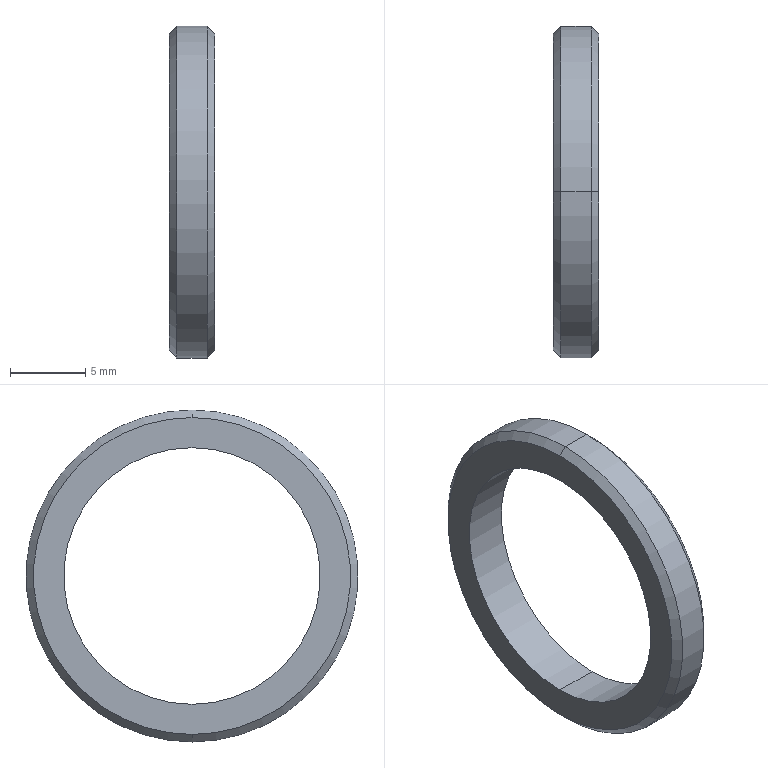Part | STEP file | 0245_002_CLBUM17-22-3 | 1 solid | 10 faces | box 3 x 22 x 22 mm | volume 442.441 mm3 | cone 4 | cylinder 4 | plane 2 | commonest cylinder face diameters 17 x2 22 x2
STEP:
#1=CARTESIAN_POINT('',(0.,0.,0.));
#2=DIRECTION('',(0.,0.,1.));
#3=DIRECTION('',(1.,0.,0.));
#4=AXIS2_PLACEMENT_3D('',#1,#2,#3);
#5=CARTESIAN_POINT('',(0.,0.,10.5));
#6=VERTEX_POINT('',#5);
#7=CARTESIAN_POINT('',(0.,0.,-10.5));
#8=VERTEX_POINT('',#7);
#9=CARTESIAN_POINT('',(0.,0.,0.));
#10=DIRECTION('',(-1.,0.,0.));
#11=DIRECTION('',(0.,0.,-1.));
#12=AXIS2_PLACEMENT_3D('',#9,#10,#11);
#13=CIRCLE('',#12,10.5);
#14=CARTESIAN_POINT('',(0.5,0.,0.));
#15=DIRECTION('',(1.,0.,0.));
#16=DIRECTION('',(0.,0.,-1.));
#17=AXIS2_PLACEMENT_3D('',#14,#15,#16);
#18=CONICAL_SURFACE('',#17,11.,0.7854);
#19=CARTESIAN_POINT('',(6.283,-0.5));
#20=DIRECTION('',(-1.,0.));
#21=VECTOR('',#20,1.);
#22=LINE('',#19,#21);
#23=(GEOMETRIC_REPRESENTATION_CONTEXT(2)PARAMETRIC_REPRESENTATION_CONTEXT()REPRESENTATION_CONTEXT('',''));
#24=DEFINITIONAL_REPRESENTATION('',(#22),#23);
#25=PCURVE('',#18,#24);
#26=CARTESIAN_POINT('',(0.,9.5,0.));
#27=DIRECTION('',(-1.,0.,0.));
#28=DIRECTION('',(0.,0.,1.));
#29=AXIS2_PLACEMENT_3D('',#26,#27,#28);
#30=PLANE('',#29);
#31=CARTESIAN_POINT('',(0.,-9.5));
#32=DIRECTION('',(-1.,0.));
#33=AXIS2_PLACEMENT_2D('',#31,#32);
#34=CIRCLE('',#33,10.5);
#35=(GEOMETRIC_REPRESENTATION_CONTEXT(2)PARAMETRIC_REPRESENTATION_CONTEXT()REPRESENTATION_CONTEXT('',''));
#36=DEFINITIONAL_REPRESENTATION('',(#34),#35);
#37=PCURVE('',#30,#36);
#38=SURFACE_CURVE('',#13,(#25,#37),.PCURVE_S1.);
#39=EDGE_CURVE('',#6,#8,#38,.T.);
#40=ORIENTED_EDGE('',*,*,#39,.F.);
#41=CARTESIAN_POINT('',(0.5,0.,11.));
#42=VERTEX_POINT('',#41);
#43=CARTESIAN_POINT('',(0.5,0.,11.));
#44=DIRECTION('',(0.7071,0.,0.7071));
#45=VECTOR('',#44,1.);
#46=LINE('',#43,#45);
#47=CARTESIAN_POINT('',(3.142,0.));
#48=DIRECTION('',(0.,1.));
#49=VECTOR('',#48,1.);
#50=LINE('',#47,#49);
#51=(GEOMETRIC_REPRESENTATION_CONTEXT(2)PARAMETRIC_REPRESENTATION_CONTEXT()REPRESENTATION_CONTEXT('',''));
#52=DEFINITIONAL_REPRESENTATION('',(#50),#51);
#53=PCURVE('',#18,#52);
#54=CARTESIAN_POINT('',(0.5,0.,0.));
#55=DIRECTION('',(1.,0.,0.));
#56=DIRECTION('',(0.,0.,-1.));
#57=AXIS2_PLACEMENT_3D('',#54,#55,#56);
#58=CONICAL_SURFACE('',#57,11.,0.7854);
#59=CARTESIAN_POINT('',(3.142,0.));
#60=DIRECTION('',(0.,1.));
#61=VECTOR('',#60,1.);
#62=LINE('',#59,#61);
#63=(GEOMETRIC_REPRESENTATION_CONTEXT(2)PARAMETRIC_REPRESENTATION_CONTEXT()REPRESENTATION_CONTEXT('',''));
#64=DEFINITIONAL_REPRESENTATION('',(#62),#63);
#65=PCURVE('',#58,#64);
#66=SURFACE_CURVE('',#46,(#53,#65),.PCURVE_S1.);
#67=EDGE_CURVE('',#6,#42,#66,.T.);
#68=ORIENTED_EDGE('',*,*,#67,.T.);
#69=CARTESIAN_POINT('',(0.5,0.,-11.));
#70=VERTEX_POINT('',#69);
#71=CARTESIAN_POINT('',(0.5,0.,0.));
#72=DIRECTION('',(-1.,0.,0.));
#73=DIRECTION('',(0.,1.,0.));
#74=AXIS2_PLACEMENT_3D('',#71,#72,#73);
#75=CIRCLE('',#74,11.);
#76=CARTESIAN_POINT('',(7.854,0.));
#77=DIRECTION('',(-1.,0.));
#78=VECTOR('',#77,1.);
#79=LINE('',#76,#78);
#80=(GEOMETRIC_REPRESENTATION_CONTEXT(2)PARAMETRIC_REPRESENTATION_CONTEXT()REPRESENTATION_CONTEXT('',''));
#81=DEFINITIONAL_REPRESENTATION('',(#79),#80);
#82=PCURVE('',#18,#81);
#83=CARTESIAN_POINT('',(1.5,0.,0.));
#84=DIRECTION('',(1.,0.,0.));
#85=DIRECTION('',(0.,0.,-1.));
#86=AXIS2_PLACEMENT_3D('',#83,#84,#85);
#87=CYLINDRICAL_SURFACE('',#86,11.);
#88=CARTESIAN_POINT('',(7.854,-1.));
#89=DIRECTION('',(-1.,0.));
#90=VECTOR('',#89,1.);
#91=LINE('',#88,#90);
#92=(GEOMETRIC_REPRESENTATION_CONTEXT(2)PARAMETRIC_REPRESENTATION_CONTEXT()REPRESENTATION_CONTEXT('',''));
#93=DEFINITIONAL_REPRESENTATION('',(#91),#92);
#94=PCURVE('',#87,#93);
#95=SURFACE_CURVE('',#75,(#82,#94),.PCURVE_S1.);
#96=EDGE_CURVE('',#42,#70,#95,.T.);
#97=ORIENTED_EDGE('',*,*,#96,.T.);
#98=CARTESIAN_POINT('',(0.5,0.,-11.));
#99=DIRECTION('',(0.7071,0.,-0.7071));
#100=VECTOR('',#99,1.);
#101=LINE('',#98,#100);
#102=CARTESIAN_POINT('',(0.,0.));
#103=DIRECTION('',(0.,1.));
#104=VECTOR('',#103,1.);
#105=LINE('',#102,#104);
#106=(GEOMETRIC_REPRESENTATION_CONTEXT(2)PARAMETRIC_REPRESENTATION_CONTEXT()REPRESENTATION_CONTEXT('',''));
#107=DEFINITIONAL_REPRESENTATION('',(#105),#106);
#108=PCURVE('',#18,#107);
#109=CARTESIAN_POINT('',(6.283,0.));
#110=DIRECTION('',(0.,1.));
#111=VECTOR('',#110,1.);
#112=LINE('',#109,#111);
#113=(GEOMETRIC_REPRESENTATION_CONTEXT(2)PARAMETRIC_REPRESENTATION_CONTEXT()REPRESENTATION_CONTEXT('',''));
#114=DEFINITIONAL_REPRESENTATION('',(#112),#113);
#115=PCURVE('',#58,#114);
#116=SURFACE_CURVE('',#101,(#108,#115),.PCURVE_S1.);
#117=EDGE_CURVE('',#8,#70,#116,.T.);
#118=ORIENTED_EDGE('',*,*,#117,.F.);
#119=EDGE_LOOP('',(#40,#68,#97,#118));
#120=FACE_BOUND('',#119,.T.);
#121=ADVANCED_FACE('',(#120),#18,.T.);
#122=CARTESIAN_POINT('',(0.,0.,-8.5));
#123=VERTEX_POINT('',#122);
#124=CARTESIAN_POINT('',(3.,0.,-8.5));
#125=VERTEX_POINT('',#124);
#126=CARTESIAN_POINT('',(1.5,0.,-8.5));
#127=DIRECTION('',(1.,0.,0.));
#128=VECTOR('',#127,1.);
#129=LINE('',#126,#128);
#130=CARTESIAN_POINT('',(1.5,0.,0.));
#131=DIRECTION('',(1.,0.,0.));
#132=DIRECTION('',(0.,0.,-1.));
#133=AXIS2_PLACEMENT_3D('',#130,#131,#132);
#134=CYLINDRICAL_SURFACE('',#133,8.5);
#135=CARTESIAN_POINT('',(6.283,0.));
#136=DIRECTION('',(0.,1.));
#137=VECTOR('',#136,1.);
#138=LINE('',#135,#137);
#139=(GEOMETRIC_REPRESENTATION_CONTEXT(2)PARAMETRIC_REPRESENTATION_CONTEXT()REPRESENTATION_CONTEXT('',''));
#140=DEFINITIONAL_REPRESENTATION('',(#138),#139);
#141=PCURVE('',#134,#140);
#142=CARTESIAN_POINT('',(1.5,0.,0.));
#143=DIRECTION('',(1.,0.,0.));
#144=DIRECTION('',(0.,0.,-1.));
#145=AXIS2_PLACEMENT_3D('',#142,#143,#144);
#146=CYLINDRICAL_SURFACE('',#145,8.5);
#147=CARTESIAN_POINT('',(0.,0.));
#148=DIRECTION('',(0.,1.));
#149=VECTOR('',#148,1.);
#150=LINE('',#147,#149);
#151=(GEOMETRIC_REPRESENTATION_CONTEXT(2)PARAMETRIC_REPRESENTATION_CONTEXT()REPRESENTATION_CONTEXT('',''));
#152=DEFINITIONAL_REPRESENTATION('',(#150),#151);
#153=PCURVE('',#146,#152);
#154=SURFACE_CURVE('',#129,(#141,#153),.PCURVE_S1.);
#155=EDGE_CURVE('',#123,#125,#154,.T.);
#156=ORIENTED_EDGE('',*,*,#155,.T.);
#157=CARTESIAN_POINT('',(3.,0.,8.5));
#158=VERTEX_POINT('',#157);
#159=CARTESIAN_POINT('',(3.,0.,0.));
#160=DIRECTION('',(-1.,0.,0.));
#161=DIRECTION('',(0.,0.,-1.));
#162=AXIS2_PLACEMENT_3D('',#159,#160,#161);
#163=CIRCLE('',#162,8.5);
#164=CARTESIAN_POINT('',(6.283,1.5));
#165=DIRECTION('',(-1.,0.));
#166=VECTOR('',#165,1.);
#167=LINE('',#164,#166);
#168=(GEOMETRIC_REPRESENTATION_CONTEXT(2)PARAMETRIC_REPRESENTATION_CONTEXT()REPRESENTATION_CONTEXT('',''));
#169=DEFINITIONAL_REPRESENTATION('',(#167),#168);
#170=PCURVE('',#134,#169);
#171=CARTESIAN_POINT('',(3.,9.5,0.));
#172=DIRECTION('',(1.,0.,0.));
#173=DIRECTION('',(0.,0.,-1.));
#174=AXIS2_PLACEMENT_3D('',#171,#172,#173);
#175=PLANE('',#174);
#176=CARTESIAN_POINT('',(8.5,-9.5));
#177=CARTESIAN_POINT('',(8.5,-24.222));
#178=CARTESIAN_POINT('',(-4.25,-16.861));
#179=CARTESIAN_POINT('',(-17.,-9.5));
#180=CARTESIAN_POINT('',(-4.25,-2.139));
#181=CARTESIAN_POINT('',(8.5,5.222));
#182=CARTESIAN_POINT('',(8.5,-9.5));
#183=(BOUNDED_CURVE()B_SPLINE_CURVE(2,(#176,#177,#178,#179,#180,#181,#182),.UNSPECIFIED.,.T.,.F.)B_SPLINE_CURVE_WITH_KNOTS((1,2,2,2,2,1),(-2.094,0.,2.094,4.189,6.283,8.378),.UNSPECIFIED.)CURVE()GEOMETRIC_REPRESENTATION_ITEM()RATIONAL_B_SPLINE_CURVE((1.,0.5,1.,0.5,1.,0.5,1.))REPRESENTATION_ITEM(''));
#184=(GEOMETRIC_REPRESENTATION_CONTEXT(2)PARAMETRIC_REPRESENTATION_CONTEXT()REPRESENTATION_CONTEXT('',''));
#185=DEFINITIONAL_REPRESENTATION('',(#183),#184);
#186=PCURVE('',#175,#185);
#187=SURFACE_CURVE('',#163,(#170,#186),.PCURVE_S1.);
#188=EDGE_CURVE('',#125,#158,#187,.T.);
#189=ORIENTED_EDGE('',*,*,#188,.T.);
#190=CARTESIAN_POINT('',(0.,0.,8.5));
#191=VERTEX_POINT('',#190);
#192=CARTESIAN_POINT('',(1.5,0.,8.5));
#193=DIRECTION('',(1.,0.,0.));
#194=VECTOR('',#193,1.);
#195=LINE('',#192,#194);
#196=CARTESIAN_POINT('',(3.142,0.));
#197=DIRECTION('',(0.,1.));
#198=VECTOR('',#197,1.);
#199=LINE('',#196,#198);
#200=(GEOMETRIC_REPRESENTATION_CONTEXT(2)PARAMETRIC_REPRESENTATION_CONTEXT()REPRESENTATION_CONTEXT('',''));
#201=DEFINITIONAL_REPRESENTATION('',(#199),#200);
#202=PCURVE('',#134,#201);
#203=CARTESIAN_POINT('',(3.142,0.));
#204=DIRECTION('',(0.,1.));
#205=VECTOR('',#204,1.);
#206=LINE('',#203,#205);
#207=(GEOMETRIC_REPRESENTATION_CONTEXT(2)PARAMETRIC_REPRESENTATION_CONTEXT()REPRESENTATION_CONTEXT('',''));
#208=DEFINITIONAL_REPRESENTATION('',(#206),#207);
#209=PCURVE('',#146,#208);
#210=SURFACE_CURVE('',#195,(#202,#209),.PCURVE_S1.);
#211=EDGE_CURVE('',#191,#158,#210,.T.);
#212=ORIENTED_EDGE('',*,*,#211,.F.);
#213=CARTESIAN_POINT('',(0.,0.,0.));
#214=DIRECTION('',(1.,0.,0.));
#215=DIRECTION('',(0.,0.,-1.));
#216=AXIS2_PLACEMENT_3D('',#213,#214,#215);
#217=CIRCLE('',#216,8.5);
#218=CARTESIAN_POINT('',(0.,-1.5));
#219=DIRECTION('',(1.,0.));
#220=VECTOR('',#219,1.);
#221=LINE('',#218,#220);
#222=(GEOMETRIC_REPRESENTATION_CONTEXT(2)PARAMETRIC_REPRESENTATION_CONTEXT()REPRESENTATION_CONTEXT('',''));
#223=DEFINITIONAL_REPRESENTATION('',(#221),#222);
#224=PCURVE('',#134,#223);
#225=CARTESIAN_POINT('',(-8.5,-9.5));
#226=CARTESIAN_POINT('',(-8.5,5.222));
#227=CARTESIAN_POINT('',(4.25,-2.139));
#228=CARTESIAN_POINT('',(17.,-9.5));
#229=CARTESIAN_POINT('',(4.25,-16.861));
#230=CARTESIAN_POINT('',(-8.5,-24.222));
#231=CARTESIAN_POINT('',(-8.5,-9.5));
#232=(BOUNDED_CURVE()B_SPLINE_CURVE(2,(#225,#226,#227,#228,#229,#230,#231),.UNSPECIFIED.,.T.,.F.)B_SPLINE_CURVE_WITH_KNOTS((1,2,2,2,2,1),(-2.094,0.,2.094,4.189,6.283,8.378),.UNSPECIFIED.)CURVE()GEOMETRIC_REPRESENTATION_ITEM()RATIONAL_B_SPLINE_CURVE((1.,0.5,1.,0.5,1.,0.5,1.))REPRESENTATION_ITEM(''));
#233=(GEOMETRIC_REPRESENTATION_CONTEXT(2)PARAMETRIC_REPRESENTATION_CONTEXT()REPRESENTATION_CONTEXT('',''));
#234=DEFINITIONAL_REPRESENTATION('',(#232),#233);
#235=PCURVE('',#30,#234);
#236=SURFACE_CURVE('',#217,(#224,#235),.PCURVE_S1.);
#237=EDGE_CURVE('',#191,#123,#236,.T.);
#238=ORIENTED_EDGE('',*,*,#237,.T.);
#239=EDGE_LOOP('',(#156,#189,#212,#238));
#240=FACE_BOUND('',#239,.F.);
#241=ADVANCED_FACE('',(#240),#134,.F.);
#242=ORIENTED_EDGE('',*,*,#96,.F.);
#243=CARTESIAN_POINT('',(2.5,0.,11.));
#244=VERTEX_POINT('',#243);
#245=CARTESIAN_POINT('',(1.5,0.,11.));
#246=DIRECTION('',(1.,0.,0.));
#247=VECTOR('',#246,1.);
#248=LINE('',#245,#247);
#249=CARTESIAN_POINT('',(3.142,0.));
#250=DIRECTION('',(0.,1.));
#251=VECTOR('',#250,1.);
#252=LINE('',#249,#251);
#253=(GEOMETRIC_REPRESENTATION_CONTEXT(2)PARAMETRIC_REPRESENTATION_CONTEXT()REPRESENTATION_CONTEXT('',''));
#254=DEFINITIONAL_REPRESENTATION('',(#252),#253);
#255=PCURVE('',#87,#254);
#256=CARTESIAN_POINT('',(1.5,0.,0.));
#257=DIRECTION('',(1.,0.,0.));
#258=DIRECTION('',(0.,0.,-1.));
#259=AXIS2_PLACEMENT_3D('',#256,#257,#258);
#260=CYLINDRICAL_SURFACE('',#259,11.);
#261=CARTESIAN_POINT('',(3.142,0.));
#262=DIRECTION('',(0.,1.));
#263=VECTOR('',#262,1.);
#264=LINE('',#261,#263);
#265=(GEOMETRIC_REPRESENTATION_CONTEXT(2)PARAMETRIC_REPRESENTATION_CONTEXT()REPRESENTATION_CONTEXT('',''));
#266=DEFINITIONAL_REPRESENTATION('',(#264),#265);
#267=PCURVE('',#260,#266);
#268=SURFACE_CURVE('',#248,(#255,#267),.PCURVE_S1.);
#269=EDGE_CURVE('',#42,#244,#268,.T.);
#270=ORIENTED_EDGE('',*,*,#269,.T.);
#271=CARTESIAN_POINT('',(2.5,0.,-11.));
#272=VERTEX_POINT('',#271);
#273=CARTESIAN_POINT('',(2.5,0.,0.));
#274=DIRECTION('',(-1.,0.,0.));
#275=DIRECTION('',(0.,0.,-1.));
#276=AXIS2_PLACEMENT_3D('',#273,#274,#275);
#277=CIRCLE('',#276,11.);
#278=CARTESIAN_POINT('',(6.283,1.));
#279=DIRECTION('',(-1.,0.));
#280=VECTOR('',#279,1.);
#281=LINE('',#278,#280);
#282=(GEOMETRIC_REPRESENTATION_CONTEXT(2)PARAMETRIC_REPRESENTATION_CONTEXT()REPRESENTATION_CONTEXT('',''));
#283=DEFINITIONAL_REPRESENTATION('',(#281),#282);
#284=PCURVE('',#87,#283);
#285=CARTESIAN_POINT('',(2.5,0.,0.));
#286=DIRECTION('',(-1.,0.,0.));
#287=DIRECTION('',(0.,0.,1.));
#288=AXIS2_PLACEMENT_3D('',#285,#286,#287);
#289=CONICAL_SURFACE('',#288,11.,0.7854);
#290=CARTESIAN_POINT('',(-3.142,0.));
#291=DIRECTION('',(1.,0.));
#292=VECTOR('',#291,1.);
#293=LINE('',#290,#292);
#294=(GEOMETRIC_REPRESENTATION_CONTEXT(2)PARAMETRIC_REPRESENTATION_CONTEXT()REPRESENTATION_CONTEXT('',''));
#295=DEFINITIONAL_REPRESENTATION('',(#293),#294);
#296=PCURVE('',#289,#295);
#297=SURFACE_CURVE('',#277,(#284,#296),.PCURVE_S1.);
#298=EDGE_CURVE('',#244,#272,#297,.T.);
#299=ORIENTED_EDGE('',*,*,#298,.T.);
#300=CARTESIAN_POINT('',(1.5,0.,-11.));
#301=DIRECTION('',(1.,0.,0.));
#302=VECTOR('',#301,1.);
#303=LINE('',#300,#302);
#304=CARTESIAN_POINT('',(0.,0.));
#305=DIRECTION('',(0.,1.));
#306=VECTOR('',#305,1.);
#307=LINE('',#304,#306);
#308=(GEOMETRIC_REPRESENTATION_CONTEXT(2)PARAMETRIC_REPRESENTATION_CONTEXT()REPRESENTATION_CONTEXT('',''));
#309=DEFINITIONAL_REPRESENTATION('',(#307),#308);
#310=PCURVE('',#87,#309);
#311=CARTESIAN_POINT('',(6.283,0.));
#312=DIRECTION('',(0.,1.));
#313=VECTOR('',#312,1.);
#314=LINE('',#311,#313);
#315=(GEOMETRIC_REPRESENTATION_CONTEXT(2)PARAMETRIC_REPRESENTATION_CONTEXT()REPRESENTATION_CONTEXT('',''));
#316=DEFINITIONAL_REPRESENTATION('',(#314),#315);
#317=PCURVE('',#260,#316);
#318=SURFACE_CURVE('',#303,(#310,#317),.PCURVE_S1.);
#319=EDGE_CURVE('',#70,#272,#318,.T.);
#320=ORIENTED_EDGE('',*,*,#319,.F.);
#321=EDGE_LOOP('',(#242,#270,#299,#320));
#322=FACE_BOUND('',#321,.T.);
#323=ADVANCED_FACE('',(#322),#87,.T.);
#324=CARTESIAN_POINT('',(3.,0.,-10.5));
#325=VERTEX_POINT('',#324);
#326=CARTESIAN_POINT('',(3.,0.,10.5));
#327=VERTEX_POINT('',#326);
#328=CARTESIAN_POINT('',(3.,0.,0.));
#329=DIRECTION('',(1.,0.,0.));
#330=DIRECTION('',(0.,0.,1.));
#331=AXIS2_PLACEMENT_3D('',#328,#329,#330);
#332=CIRCLE('',#331,10.5);
#333=CARTESIAN_POINT('',(6.283,-0.5));
#334=DIRECTION('',(-1.,0.));
#335=VECTOR('',#334,1.);
#336=LINE('',#333,#335);
#337=(GEOMETRIC_REPRESENTATION_CONTEXT(2)PARAMETRIC_REPRESENTATION_CONTEXT()REPRESENTATION_CONTEXT('',''));
#338=DEFINITIONAL_REPRESENTATION('',(#336),#337);
#339=PCURVE('',#289,#338);
#340=CARTESIAN_POINT('',(0.,-9.5));
#341=DIRECTION('',(-1.,0.));
#342=AXIS2_PLACEMENT_2D('',#340,#341);
#343=CIRCLE('',#342,10.5);
#344=(GEOMETRIC_REPRESENTATION_CONTEXT(2)PARAMETRIC_REPRESENTATION_CONTEXT()REPRESENTATION_CONTEXT('',''));
#345=DEFINITIONAL_REPRESENTATION('',(#343),#344);
#346=PCURVE('',#175,#345);
#347=SURFACE_CURVE('',#332,(#339,#346),.PCURVE_S1.);
#348=EDGE_CURVE('',#325,#327,#347,.T.);
#349=ORIENTED_EDGE('',*,*,#348,.F.);
#350=CARTESIAN_POINT('',(2.5,0.,-11.));
#351=DIRECTION('',(-0.7071,0.,-0.7071));
#352=VECTOR('',#351,1.);
#353=LINE('',#350,#352);
#354=CARTESIAN_POINT('',(3.142,0.));
#355=DIRECTION('',(0.,1.));
#356=VECTOR('',#355,1.);
#357=LINE('',#354,#356);
#358=(GEOMETRIC_REPRESENTATION_CONTEXT(2)PARAMETRIC_REPRESENTATION_CONTEXT()REPRESENTATION_CONTEXT('',''));
#359=DEFINITIONAL_REPRESENTATION('',(#357),#358);
#360=PCURVE('',#289,#359);
#361=CARTESIAN_POINT('',(2.5,0.,0.));
#362=DIRECTION('',(-1.,0.,0.));
#363=DIRECTION('',(0.,0.,1.));
#364=AXIS2_PLACEMENT_3D('',#361,#362,#363);
#365=CONICAL_SURFACE('',#364,11.,0.7854);
#366=CARTESIAN_POINT('',(3.142,0.));
#367=DIRECTION('',(0.,1.));
#368=VECTOR('',#367,1.);
#369=LINE('',#366,#368);
#370=(GEOMETRIC_REPRESENTATION_CONTEXT(2)PARAMETRIC_REPRESENTATION_CONTEXT()REPRESENTATION_CONTEXT('',''));
#371=DEFINITIONAL_REPRESENTATION('',(#369),#370);
#372=PCURVE('',#365,#371);
#373=SURFACE_CURVE('',#353,(#360,#372),.PCURVE_S1.);
#374=EDGE_CURVE('',#325,#272,#373,.T.);
#375=ORIENTED_EDGE('',*,*,#374,.T.);
#376=ORIENTED_EDGE('',*,*,#298,.F.);
#377=CARTESIAN_POINT('',(2.5,0.,11.));
#378=DIRECTION('',(-0.7071,0.,0.7071));
#379=VECTOR('',#378,1.);
#380=LINE('',#377,#379);
#381=CARTESIAN_POINT('',(0.,0.));
#382=DIRECTION('',(0.,1.));
#383=VECTOR('',#382,1.);
#384=LINE('',#381,#383);
#385=(GEOMETRIC_REPRESENTATION_CONTEXT(2)PARAMETRIC_REPRESENTATION_CONTEXT()REPRESENTATION_CONTEXT('',''));
#386=DEFINITIONAL_REPRESENTATION('',(#384),#385);
#387=PCURVE('',#289,#386);
#388=CARTESIAN_POINT('',(6.283,0.));
#389=DIRECTION('',(0.,1.));
#390=VECTOR('',#389,1.);
#391=LINE('',#388,#390);
#392=(GEOMETRIC_REPRESENTATION_CONTEXT(2)PARAMETRIC_REPRESENTATION_CONTEXT()REPRESENTATION_CONTEXT('',''));
#393=DEFINITIONAL_REPRESENTATION('',(#391),#392);
#394=PCURVE('',#365,#393);
#395=SURFACE_CURVE('',#380,(#387,#394),.PCURVE_S1.);
#396=EDGE_CURVE('',#327,#244,#395,.T.);
#397=ORIENTED_EDGE('',*,*,#396,.F.);
#398=EDGE_LOOP('',(#349,#375,#376,#397));
#399=FACE_BOUND('',#398,.T.);
#400=ADVANCED_FACE('',(#399),#289,.T.);
#401=CARTESIAN_POINT('',(0.,0.,0.));
#402=DIRECTION('',(-1.,0.,0.));
#403=DIRECTION('',(0.,0.,-1.));
#404=AXIS2_PLACEMENT_3D('',#401,#402,#403);
#405=CIRCLE('',#404,10.5);
#406=CARTESIAN_POINT('',(0.,-9.5));
#407=DIRECTION('',(-1.,0.));
#408=AXIS2_PLACEMENT_2D('',#406,#407);
#409=CIRCLE('',#408,10.5);
#410=(GEOMETRIC_REPRESENTATION_CONTEXT(2)PARAMETRIC_REPRESENTATION_CONTEXT()REPRESENTATION_CONTEXT('',''));
#411=DEFINITIONAL_REPRESENTATION('',(#409),#410);
#412=PCURVE('',#30,#411);
#413=CARTESIAN_POINT('',(6.283,-0.5));
#414=DIRECTION('',(-1.,0.));
#415=VECTOR('',#414,1.);
#416=LINE('',#413,#415);
#417=(GEOMETRIC_REPRESENTATION_CONTEXT(2)PARAMETRIC_REPRESENTATION_CONTEXT()REPRESENTATION_CONTEXT('',''));
#418=DEFINITIONAL_REPRESENTATION('',(#416),#417);
#419=PCURVE('',#58,#418);
#420=SURFACE_CURVE('',#405,(#412,#419),.PCURVE_S1.);
#421=EDGE_CURVE('',#8,#6,#420,.T.);
#422=ORIENTED_EDGE('',*,*,#421,.T.);
#423=ORIENTED_EDGE('',*,*,#39,.T.);
#424=EDGE_LOOP('',(#422,#423));
#425=FACE_BOUND('',#424,.T.);
#426=CARTESIAN_POINT('',(0.,0.,0.));
#427=DIRECTION('',(1.,0.,0.));
#428=DIRECTION('',(0.,0.,-1.));
#429=AXIS2_PLACEMENT_3D('',#426,#427,#428);
#430=CIRCLE('',#429,8.5);
#431=CARTESIAN_POINT('',(-8.5,-9.5));
#432=CARTESIAN_POINT('',(-8.5,5.222));
#433=CARTESIAN_POINT('',(4.25,-2.139));
#434=CARTESIAN_POINT('',(17.,-9.5));
#435=CARTESIAN_POINT('',(4.25,-16.861));
#436=CARTESIAN_POINT('',(-8.5,-24.222));
#437=CARTESIAN_POINT('',(-8.5,-9.5));
#438=(BOUNDED_CURVE()B_SPLINE_CURVE(2,(#431,#432,#433,#434,#435,#436,#437),.UNSPECIFIED.,.T.,.F.)B_SPLINE_CURVE_WITH_KNOTS((1,2,2,2,2,1),(-2.094,0.,2.094,4.189,6.283,8.378),.UNSPECIFIED.)CURVE()GEOMETRIC_REPRESENTATION_ITEM()RATIONAL_B_SPLINE_CURVE((1.,0.5,1.,0.5,1.,0.5,1.))REPRESENTATION_ITEM(''));
#439=(GEOMETRIC_REPRESENTATION_CONTEXT(2)PARAMETRIC_REPRESENTATION_CONTEXT()REPRESENTATION_CONTEXT('',''));
#440=DEFINITIONAL_REPRESENTATION('',(#438),#439);
#441=PCURVE('',#30,#440);
#442=CARTESIAN_POINT('',(0.,-1.5));
#443=DIRECTION('',(1.,0.));
#444=VECTOR('',#443,1.);
#445=LINE('',#442,#444);
#446=(GEOMETRIC_REPRESENTATION_CONTEXT(2)PARAMETRIC_REPRESENTATION_CONTEXT()REPRESENTATION_CONTEXT('',''));
#447=DEFINITIONAL_REPRESENTATION('',(#445),#446);
#448=PCURVE('',#146,#447);
#449=SURFACE_CURVE('',#430,(#441,#448),.PCURVE_S1.);
#450=EDGE_CURVE('',#123,#191,#449,.T.);
#451=ORIENTED_EDGE('',*,*,#450,.T.);
#452=ORIENTED_EDGE('',*,*,#237,.T.);
#453=EDGE_LOOP('',(#451,#452));
#454=FACE_BOUND('',#453,.T.);
#455=ADVANCED_FACE('',(#425,#454),#30,.T.);
#456=ORIENTED_EDGE('',*,*,#67,.F.);
#457=ORIENTED_EDGE('',*,*,#421,.F.);
#458=ORIENTED_EDGE('',*,*,#117,.T.);
#459=CARTESIAN_POINT('',(0.5,0.,0.));
#460=DIRECTION('',(-1.,0.,0.));
#461=DIRECTION('',(0.,1.,0.));
#462=AXIS2_PLACEMENT_3D('',#459,#460,#461);
#463=CIRCLE('',#462,11.);
#464=CARTESIAN_POINT('',(7.854,0.));
#465=DIRECTION('',(-1.,0.));
#466=VECTOR('',#465,1.);
#467=LINE('',#464,#466);
#468=(GEOMETRIC_REPRESENTATION_CONTEXT(2)PARAMETRIC_REPRESENTATION_CONTEXT()REPRESENTATION_CONTEXT('',''));
#469=DEFINITIONAL_REPRESENTATION('',(#467),#468);
#470=PCURVE('',#58,#469);
#471=CARTESIAN_POINT('',(7.854,-1.));
#472=DIRECTION('',(-1.,0.));
#473=VECTOR('',#472,1.);
#474=LINE('',#471,#473);
#475=(GEOMETRIC_REPRESENTATION_CONTEXT(2)PARAMETRIC_REPRESENTATION_CONTEXT()REPRESENTATION_CONTEXT('',''));
#476=DEFINITIONAL_REPRESENTATION('',(#474),#475);
#477=PCURVE('',#260,#476);
#478=SURFACE_CURVE('',#463,(#470,#477),.PCURVE_S1.);
#479=EDGE_CURVE('',#70,#42,#478,.T.);
#480=ORIENTED_EDGE('',*,*,#479,.T.);
#481=EDGE_LOOP('',(#456,#457,#458,#480));
#482=FACE_BOUND('',#481,.T.);
#483=ADVANCED_FACE('',(#482),#58,.T.);
#484=CARTESIAN_POINT('',(3.,0.,0.));
#485=DIRECTION('',(-1.,0.,0.));
#486=DIRECTION('',(0.,0.,-1.));
#487=AXIS2_PLACEMENT_3D('',#484,#485,#486);
#488=CIRCLE('',#487,8.5);
#489=CARTESIAN_POINT('',(6.283,1.5));
#490=DIRECTION('',(-1.,0.));
#491=VECTOR('',#490,1.);
#492=LINE('',#489,#491);
#493=(GEOMETRIC_REPRESENTATION_CONTEXT(2)PARAMETRIC_REPRESENTATION_CONTEXT()REPRESENTATION_CONTEXT('',''));
#494=DEFINITIONAL_REPRESENTATION('',(#492),#493);
#495=PCURVE('',#146,#494);
#496=CARTESIAN_POINT('',(8.5,-9.5));
#497=CARTESIAN_POINT('',(8.5,-24.222));
#498=CARTESIAN_POINT('',(-4.25,-16.861));
#499=CARTESIAN_POINT('',(-17.,-9.5));
#500=CARTESIAN_POINT('',(-4.25,-2.139));
#501=CARTESIAN_POINT('',(8.5,5.222));
#502=CARTESIAN_POINT('',(8.5,-9.5));
#503=(BOUNDED_CURVE()B_SPLINE_CURVE(2,(#496,#497,#498,#499,#500,#501,#502),.UNSPECIFIED.,.T.,.F.)B_SPLINE_CURVE_WITH_KNOTS((1,2,2,2,2,1),(-2.094,0.,2.094,4.189,6.283,8.378),.UNSPECIFIED.)CURVE()GEOMETRIC_REPRESENTATION_ITEM()RATIONAL_B_SPLINE_CURVE((1.,0.5,1.,0.5,1.,0.5,1.))REPRESENTATION_ITEM(''));
#504=(GEOMETRIC_REPRESENTATION_CONTEXT(2)PARAMETRIC_REPRESENTATION_CONTEXT()REPRESENTATION_CONTEXT('',''));
#505=DEFINITIONAL_REPRESENTATION('',(#503),#504);
#506=PCURVE('',#175,#505);
#507=SURFACE_CURVE('',#488,(#495,#506),.PCURVE_S1.);
#508=EDGE_CURVE('',#158,#125,#507,.T.);
#509=ORIENTED_EDGE('',*,*,#508,.T.);
#510=ORIENTED_EDGE('',*,*,#155,.F.);
#511=ORIENTED_EDGE('',*,*,#450,.T.);
#512=ORIENTED_EDGE('',*,*,#211,.T.);
#513=EDGE_LOOP('',(#509,#510,#511,#512));
#514=FACE_BOUND('',#513,.F.);
#515=ADVANCED_FACE('',(#514),#146,.F.);
#516=ORIENTED_EDGE('',*,*,#269,.F.);
#517=ORIENTED_EDGE('',*,*,#479,.F.);
#518=ORIENTED_EDGE('',*,*,#319,.T.);
#519=CARTESIAN_POINT('',(2.5,0.,0.));
#520=DIRECTION('',(-1.,0.,0.));
#521=DIRECTION('',(0.,0.,-1.));
#522=AXIS2_PLACEMENT_3D('',#519,#520,#521);
#523=CIRCLE('',#522,11.);
#524=CARTESIAN_POINT('',(6.283,1.));
#525=DIRECTION('',(-1.,0.));
#526=VECTOR('',#525,1.);
#527=LINE('',#524,#526);
#528=(GEOMETRIC_REPRESENTATION_CONTEXT(2)PARAMETRIC_REPRESENTATION_CONTEXT()REPRESENTATION_CONTEXT('',''));
#529=DEFINITIONAL_REPRESENTATION('',(#527),#528);
#530=PCURVE('',#260,#529);
#531=CARTESIAN_POINT('',(3.142,0.));
#532=DIRECTION('',(1.,0.));
#533=VECTOR('',#532,1.);
#534=LINE('',#531,#533);
#535=(GEOMETRIC_REPRESENTATION_CONTEXT(2)PARAMETRIC_REPRESENTATION_CONTEXT()REPRESENTATION_CONTEXT('',''));
#536=DEFINITIONAL_REPRESENTATION('',(#534),#535);
#537=PCURVE('',#365,#536);
#538=SURFACE_CURVE('',#523,(#530,#537),.PCURVE_S1.);
#539=EDGE_CURVE('',#272,#244,#538,.T.);
#540=ORIENTED_EDGE('',*,*,#539,.T.);
#541=EDGE_LOOP('',(#516,#517,#518,#540));
#542=FACE_BOUND('',#541,.T.);
#543=ADVANCED_FACE('',(#542),#260,.T.);
#544=ORIENTED_EDGE('',*,*,#188,.T.);
#545=ORIENTED_EDGE('',*,*,#508,.T.);
#546=EDGE_LOOP('',(#544,#545));
#547=FACE_BOUND('',#546,.T.);
#548=CARTESIAN_POINT('',(3.,0.,0.));
#549=DIRECTION('',(1.,0.,0.));
#550=DIRECTION('',(0.,0.,1.));
#551=AXIS2_PLACEMENT_3D('',#548,#549,#550);
#552=CIRCLE('',#551,10.5);
#553=CARTESIAN_POINT('',(0.,-9.5));
#554=DIRECTION('',(-1.,0.));
#555=AXIS2_PLACEMENT_2D('',#553,#554);
#556=CIRCLE('',#555,10.5);
#557=(GEOMETRIC_REPRESENTATION_CONTEXT(2)PARAMETRIC_REPRESENTATION_CONTEXT()REPRESENTATION_CONTEXT('',''));
#558=DEFINITIONAL_REPRESENTATION('',(#556),#557);
#559=PCURVE('',#175,#558);
#560=CARTESIAN_POINT('',(6.283,-0.5));
#561=DIRECTION('',(-1.,0.));
#562=VECTOR('',#561,1.);
#563=LINE('',#560,#562);
#564=(GEOMETRIC_REPRESENTATION_CONTEXT(2)PARAMETRIC_REPRESENTATION_CONTEXT()REPRESENTATION_CONTEXT('',''));
#565=DEFINITIONAL_REPRESENTATION('',(#563),#564);
#566=PCURVE('',#365,#565);
#567=SURFACE_CURVE('',#552,(#559,#566),.PCURVE_S1.);
#568=EDGE_CURVE('',#327,#325,#567,.T.);
#569=ORIENTED_EDGE('',*,*,#568,.T.);
#570=ORIENTED_EDGE('',*,*,#348,.T.);
#571=EDGE_LOOP('',(#569,#570));
#572=FACE_BOUND('',#571,.T.);
#573=ADVANCED_FACE('',(#547,#572),#175,.T.);
#574=ORIENTED_EDGE('',*,*,#374,.F.);
#575=ORIENTED_EDGE('',*,*,#568,.F.);
#576=ORIENTED_EDGE('',*,*,#396,.T.);
#577=ORIENTED_EDGE('',*,*,#539,.F.);
#578=EDGE_LOOP('',(#574,#575,#576,#577));
#579=FACE_BOUND('',#578,.T.);
#580=ADVANCED_FACE('',(#579),#365,.T.);
#581=CLOSED_SHELL('',(#121,#241,#323,#400,#455,#483,#515,#543,#573,#580));
#582=MANIFOLD_SOLID_BREP('',#581);
#583=(LENGTH_UNIT()NAMED_UNIT(*)SI_UNIT(.MILLI.,.METRE.));
#584=UNCERTAINTY_MEASURE_WITH_UNIT(LENGTH_MEASURE(0.0000001),#583,'','');
#585=(NAMED_UNIT(*)PLANE_ANGLE_UNIT()SI_UNIT($,.RADIAN.));
#586=(NAMED_UNIT(*)SI_UNIT($,.STERADIAN.)SOLID_ANGLE_UNIT());
#587=(GEOMETRIC_REPRESENTATION_CONTEXT(3)GLOBAL_UNCERTAINTY_ASSIGNED_CONTEXT((#584))GLOBAL_UNIT_ASSIGNED_CONTEXT((#583,#585,#586))REPRESENTATION_CONTEXT('',''));
#588=ADVANCED_BREP_SHAPE_REPRESENTATION('',(#4,#582),#587);